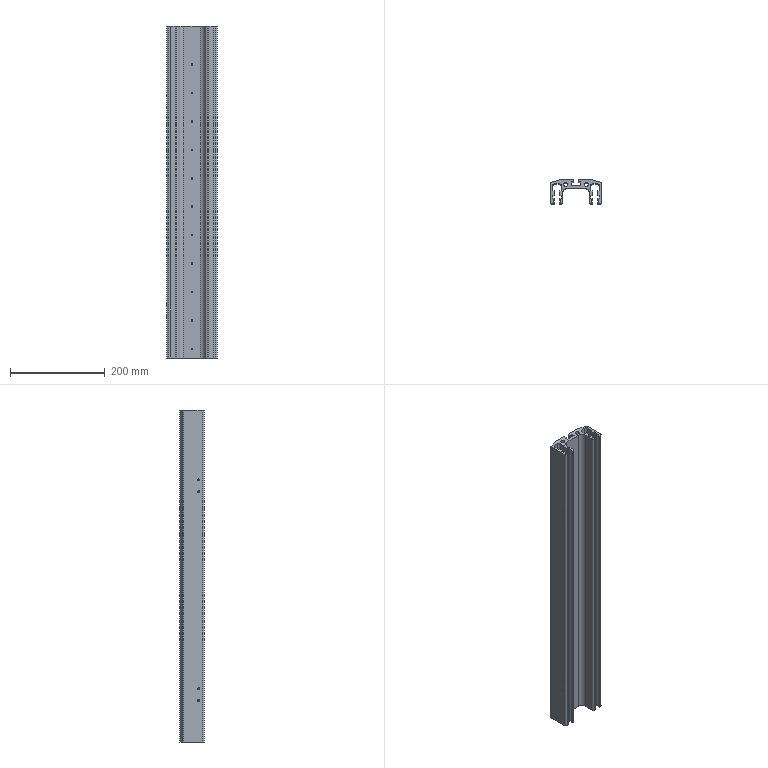Part | STEP file | Column | 1 solid | 114 faces | box 107.4 x 51 x 700 mm | volume 1396461 mm3 | plane 60 | cylinder 54 | commonest cylinder face diameters 3.3 x22 4.2 x8 8 x8 6 x6 8.7 x4 1 x2